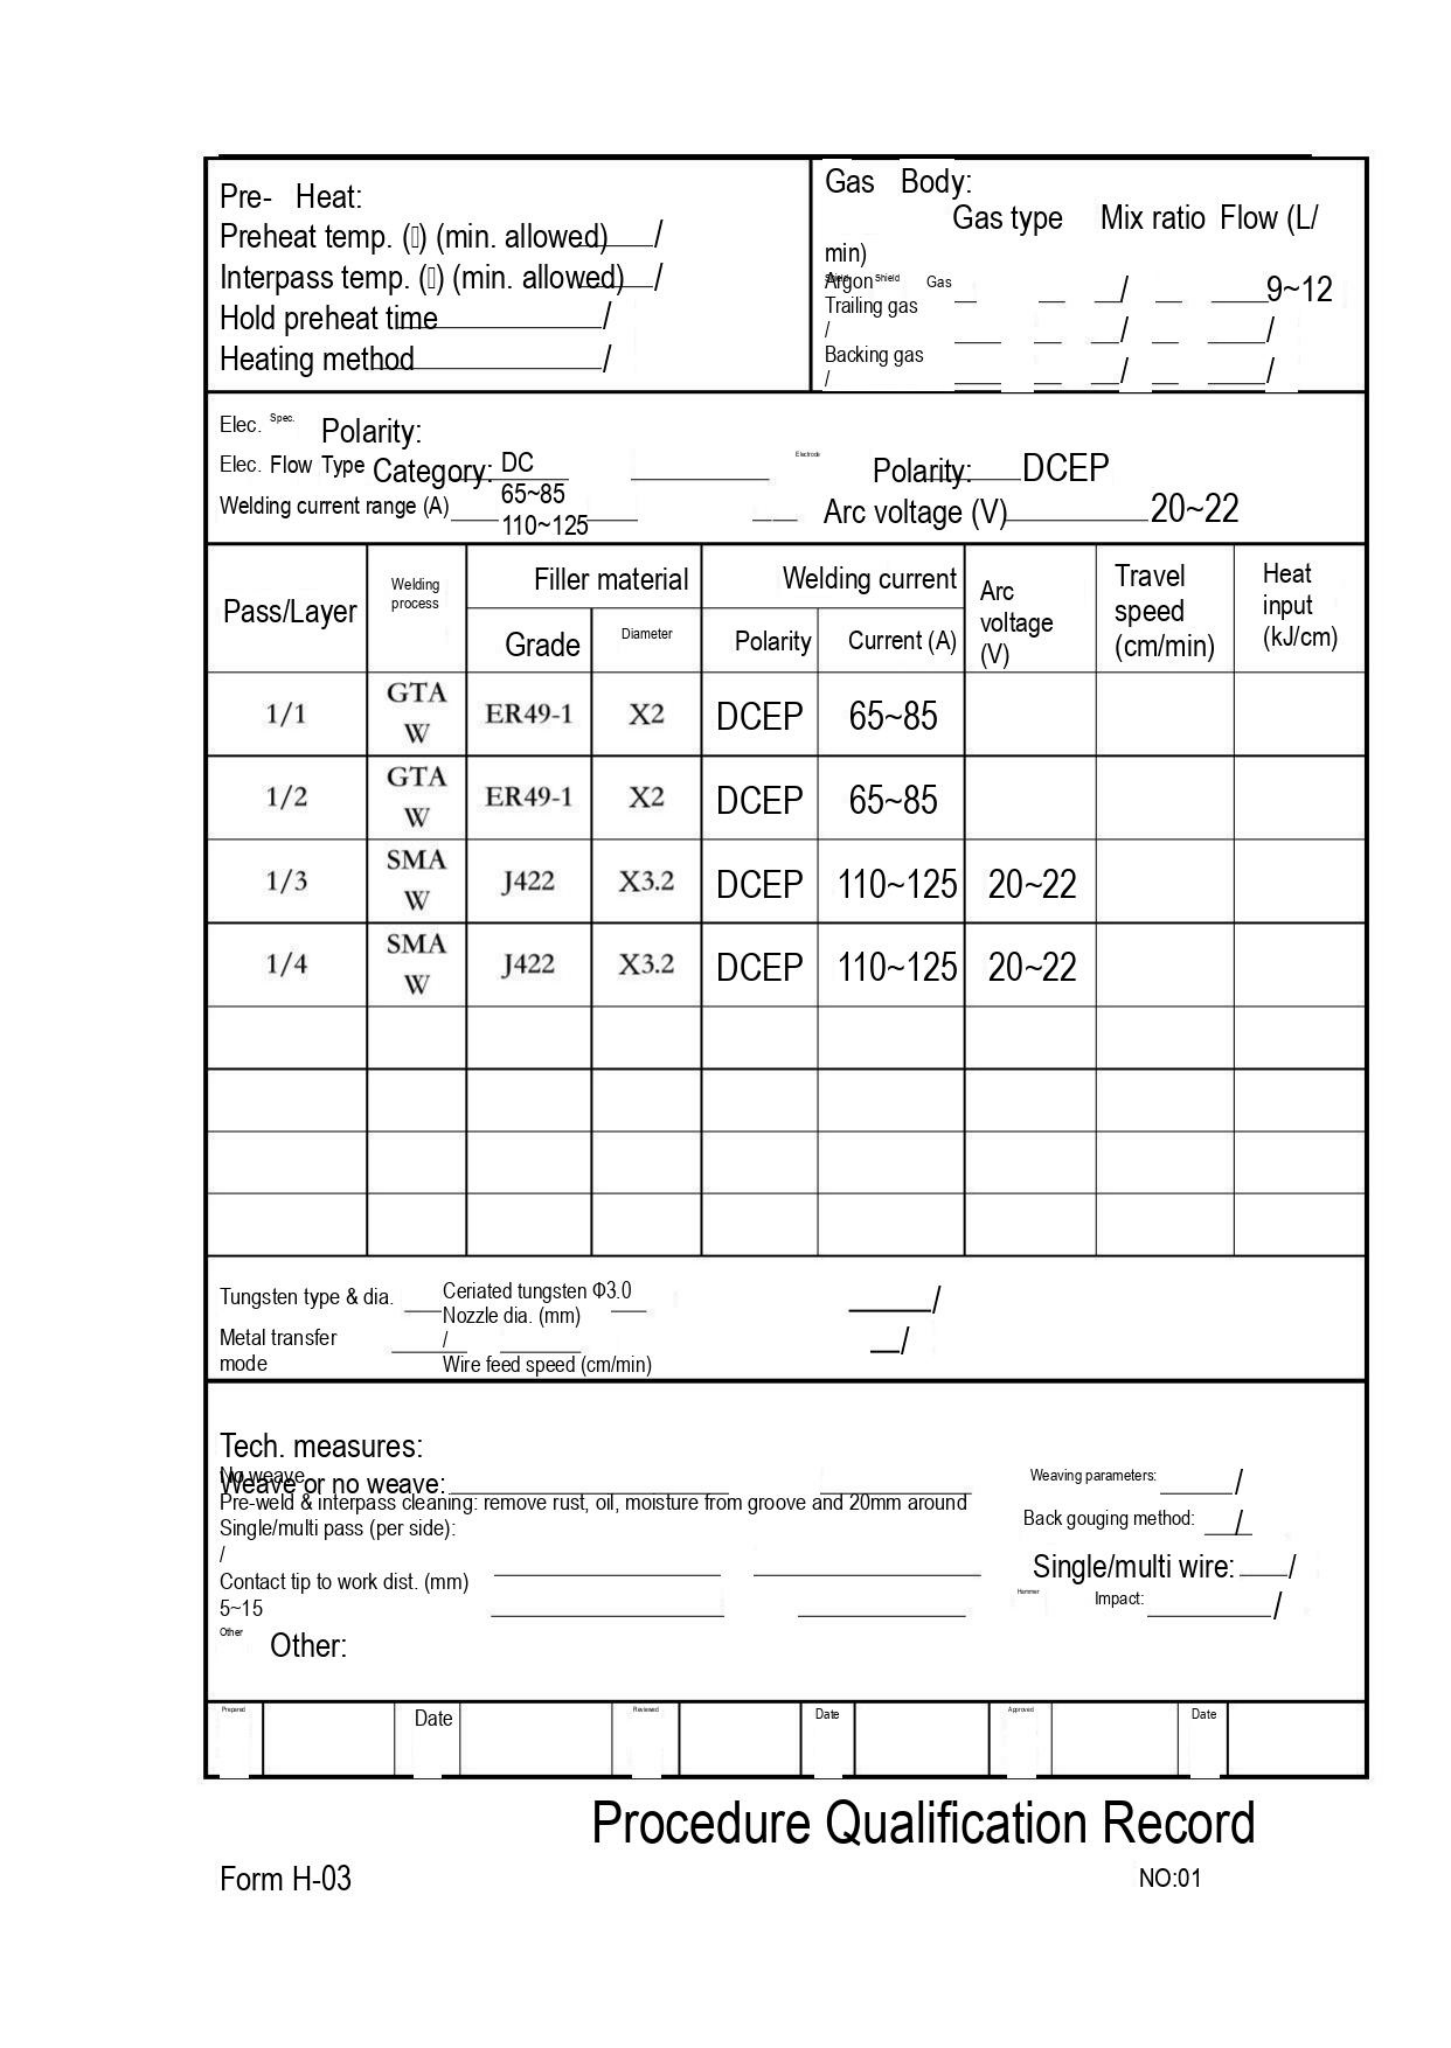Pre- Heat:
Preheat temp. (□) (min. allowed) /
Interpass temp. (□) (min. allowed) /
Hold preheat time /
Heating method /

Gas Body:
Gas type Mix ratio Flow (L/min)
Shield Argon Shield Gas / 9~12
Trailing gas / / /
Backing gas / / /

Elec. Spec. Polarity:
Elec. Flow Type Category: DC Electrode Polarity: DCEP
Welding current range (A) 65~85 110~125 Arc voltage (V) 20~22

| Pass/Layer | Welding process | Filler material Grade | Filler material Diameter | Welding current Polarity | Welding current Current (A) | Arc voltage (V) | Travel speed (cm/min) | Heat input (kJ/cm) |
|---|---|---|---|---|---|---|---|---|
| 1/1 | GTAW | ER49-1 | X2 | DCEP | 65~85 | | | |
| 1/2 | GTAW | ER49-1 | X2 | DCEP | 65~85 | | | |
| 1/3 | SMAW | J422 | X3.2 | DCEP | 110~125 | 20~22 | | |
| 1/4 | SMAW | J422 | X3.2 | DCEP | 110~125 | 20~22 | | |
| | | | | | | | | |
| | | | | | | | | |
| | | | | | | | | |
| | | | | | | | | |

Tungsten type & dia. Ceriated tungsten Φ3.0 Nozzle dia. (mm) /
Metal transfer mode / Wire feed speed (cm/min) /

Tech. measures:
No weave Weave or no weave:
Pre-weld & interpass cleaning: remove rust, oil, moisture from groove and 20mm around
Single/multi pass (per side):
/
Contact tip to work dist. (mm)
5~15
Weaving parameters: /
Back gouging method: /
Single/multi wire: /
Hammer Impact: /
Other Other:

| Prepared | | Date | | Reviewed | | Date | | Approved | | Date | |
|---|---|---|---|---|---|---|---|---|---|---|---|

Procedure Qualification Record
Form H-03
NO:01
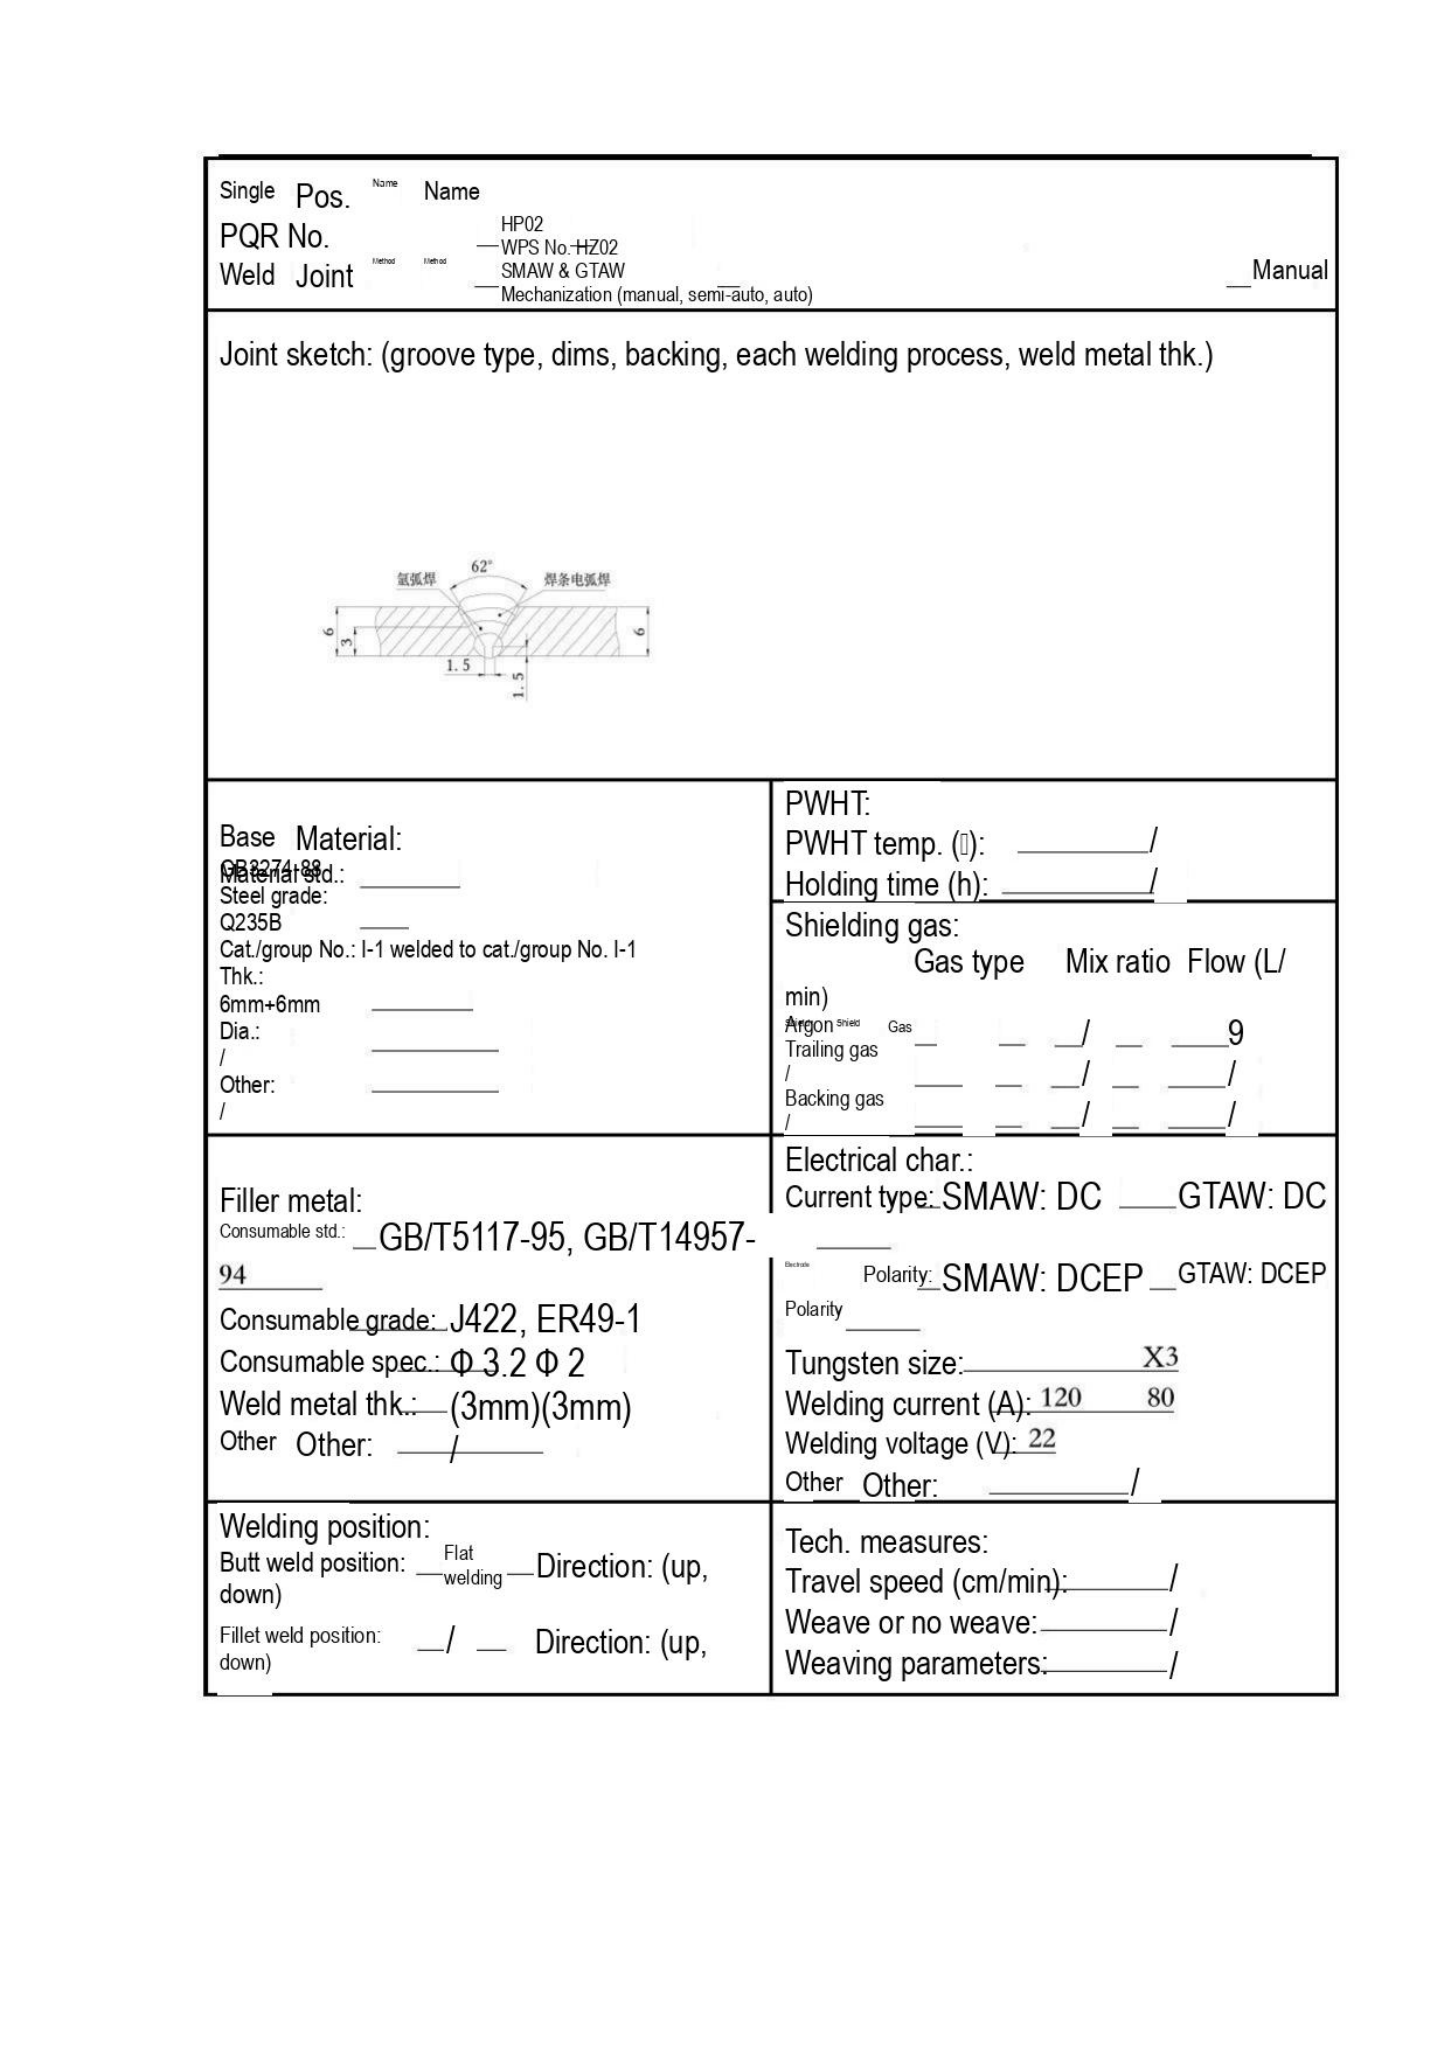Single Pos. Name Name
PQR No. HP02
WPS No. HZ02
Weld Joint Method Method SMAW & GTAW
Mechanization (manual, semi-auto, auto) Manual

Joint sketch: (groove type, dims, backing, each welding process, weld metal thk.)

氩弧焊 62° 焊条电弧焊
6 3 6
1.5 1.5

| | |
|---|---|
| Base Material:<br>Material std.: GB3274-88<br>Steel grade:<br>Q235B<br>Cat./group No.: I-1 welded to cat./group No. I-1<br>Thk.:<br>6mm+6mm<br>Dia.:<br>/<br>Other:<br>/ | PWHT:<br>PWHT temp. (): /<br>Holding time (h): / |
| | Shielding gas:<br>Gas type Mix ratio Flow (L/min)<br>Shield Gas Argon / 9<br>Trailing gas<br>/ / /<br>Backing gas<br>/ / / |
| Filler metal:<br>Consumable std.: GB/T5117-95, GB/T14957-94<br>Consumable grade: J422, ER49-1<br>Consumable spec.: Φ3.2 Φ2<br>Weld metal thk.: (3mm)(3mm)<br>Other Other: / | Electrical char.:<br>Current type: SMAW: DC GTAW: DC<br>Polarity: SMAW: DCEP GTAW: DCEP<br>Polarity<br>Tungsten size: X3<br>Welding current (A): 120 80<br>Welding voltage (V): 22<br>Other Other: / |
| Welding position:<br>Butt weld position: Flat welding Direction: (up, down)<br>Fillet weld position: / Direction: (up, down) | Tech. measures:<br>Travel speed (cm/min): /<br>Weave or no weave: /<br>Weaving parameters: / |
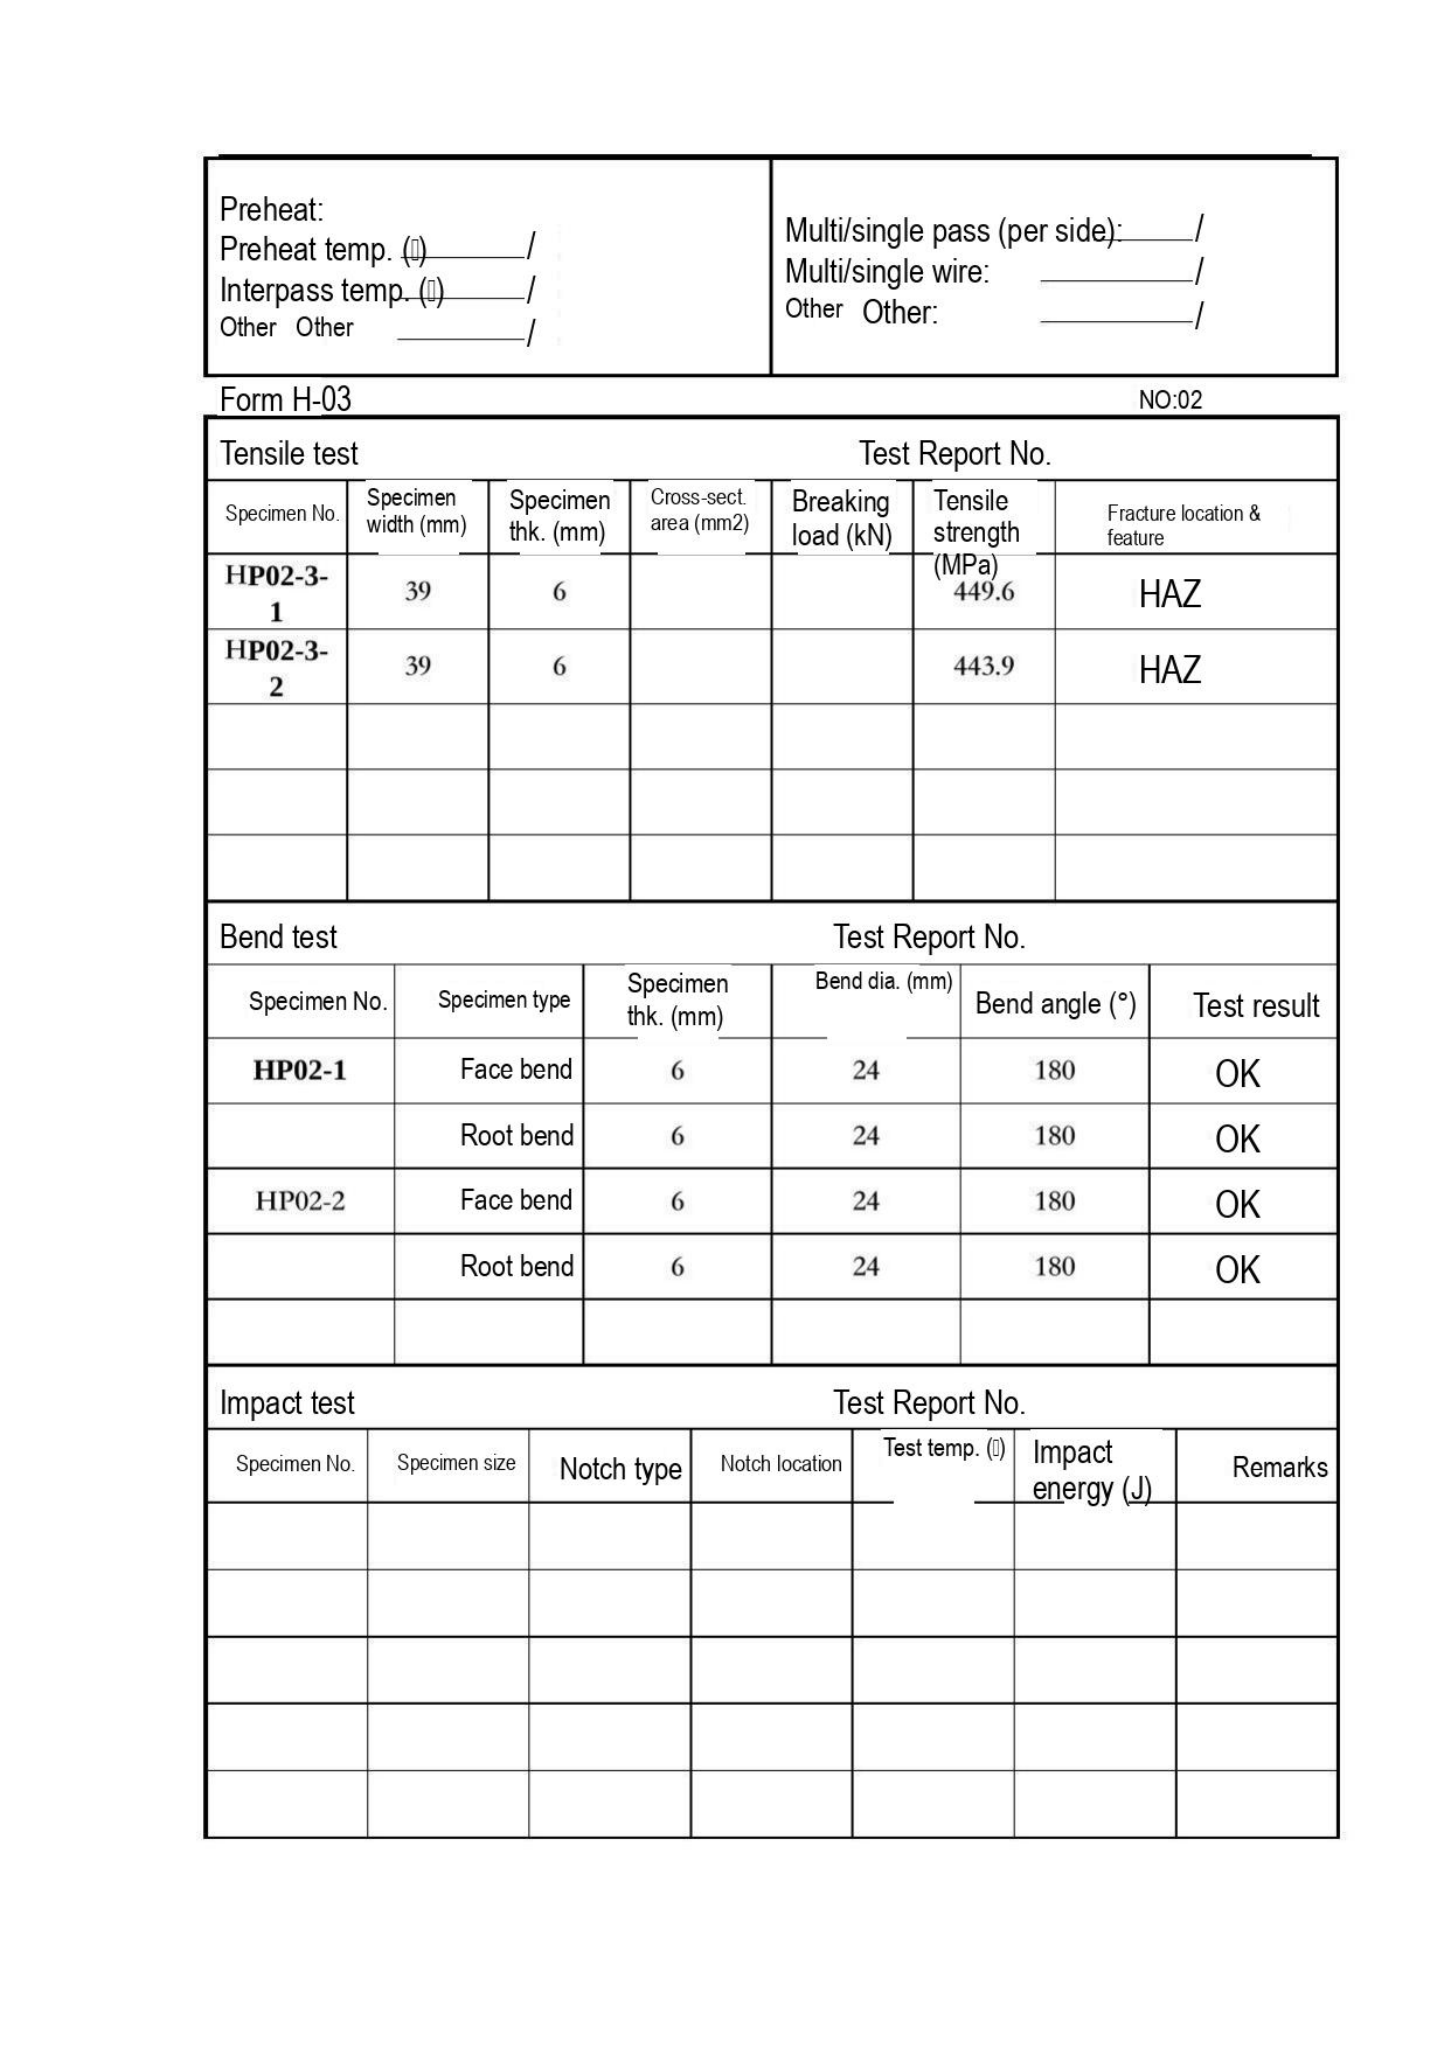Preheat:
Preheat temp. () /
Interpass temp. () /
Other Other /

Multi/single pass (per side): /
Multi/single wire: /
Other Other: /

Form H-03 NO:02

Tensile test Test Report No.

| Specimen No. | Specimen width (mm) | Specimen thk. (mm) | Cross-sect. area (mm2) | Breaking load (kN) | Tensile strength (MPa) | Fracture location & feature |
|---|---|---|---|---|---|---|
| HP02-3-1 | 39 | 6 | | | 449.6 | HAZ |
| HP02-3-2 | 39 | 6 | | | 443.9 | HAZ |
| | | | | | | |
| | | | | | | |
| | | | | | | |

Bend test Test Report No.

| Specimen No. | Specimen type | Specimen thk. (mm) | Bend dia. (mm) | Bend angle (°) | Test result |
|---|---|---|---|---|---|
| HP02-1 | Face bend | 6 | 24 | 180 | OK |
| | Root bend | 6 | 24 | 180 | OK |
| HP02-2 | Face bend | 6 | 24 | 180 | OK |
| | Root bend | 6 | 24 | 180 | OK |
| | | | | | |

Impact test Test Report No.

| Specimen No. | Specimen size | Notch type | Notch location | Test temp. () | Impact energy (J) | Remarks |
|---|---|---|---|---|---|---|
| | | | | | | |
| | | | | | | |
| | | | | | | |
| | | | | | | |
| | | | | | | |
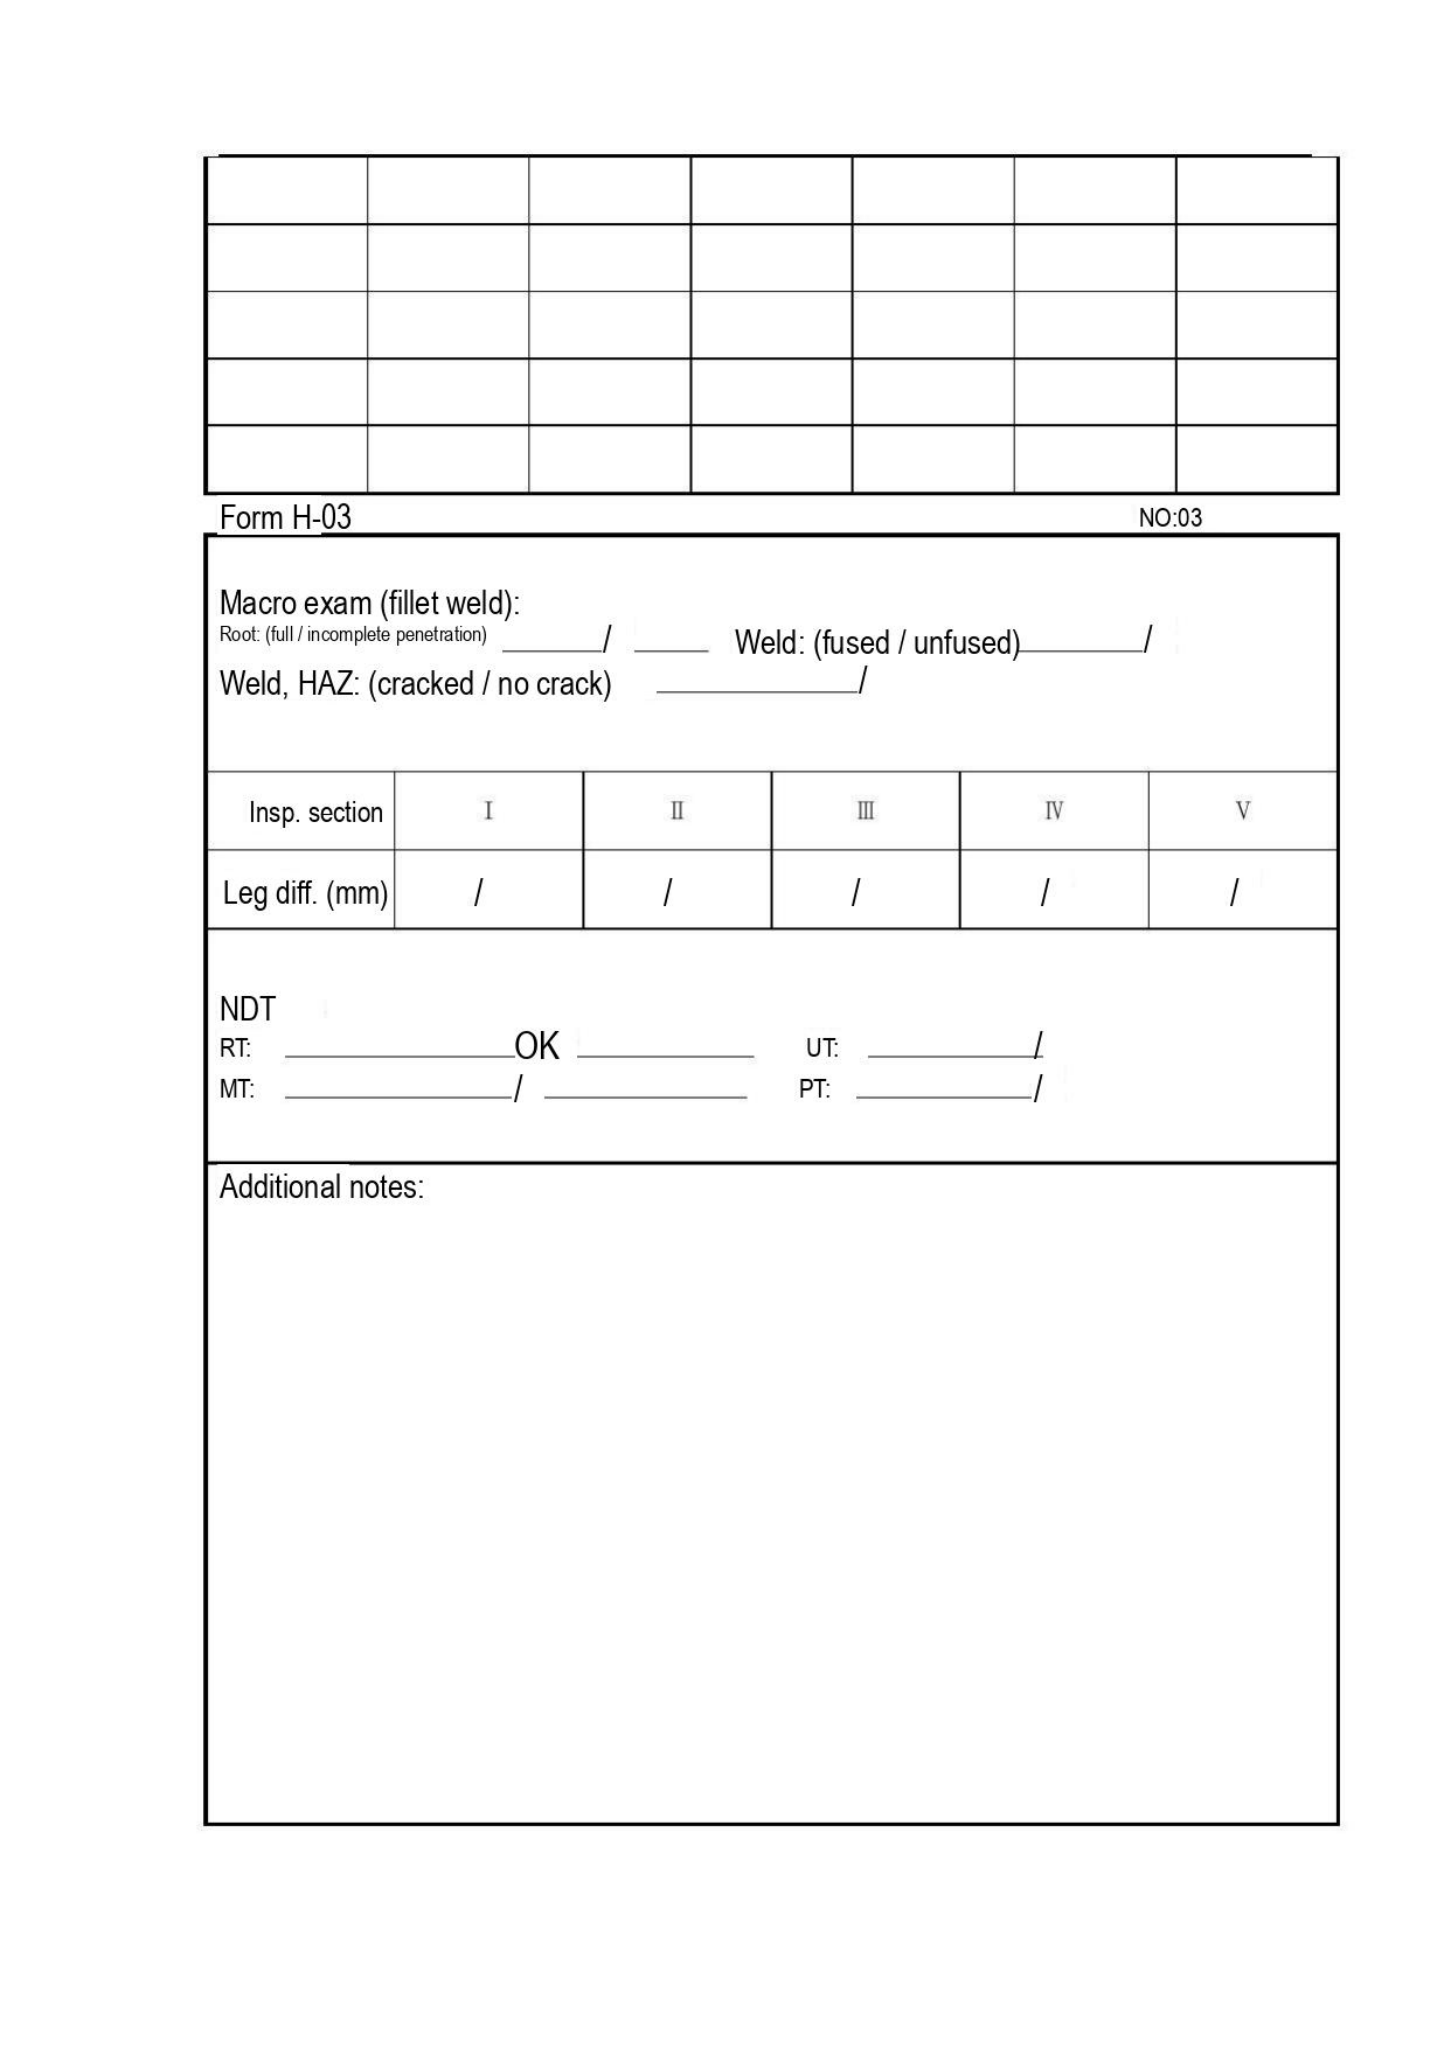|   |   |   |   |   |   |   |
|---|---|---|---|---|---|---|
|   |   |   |   |   |   |   |
|   |   |   |   |   |   |   |
|   |   |   |   |   |   |   |
|   |   |   |   |   |   |   |

Form H-03 NO:03

Macro exam (fillet weld):
Root: (full / incomplete penetration) ________/ ______ Weld: (fused / unfused)________/
Weld, HAZ: (cracked / no crack) ______________/

| Insp. section | I | II | III | IV | V |
|---|---|---|---|---|---|
| Leg diff. (mm) | / | / | / | / | / |

NDT
RT: ________________OK ______________ UT: ____________/
MT: ________________/ ______________ PT: ____________/

Additional notes:
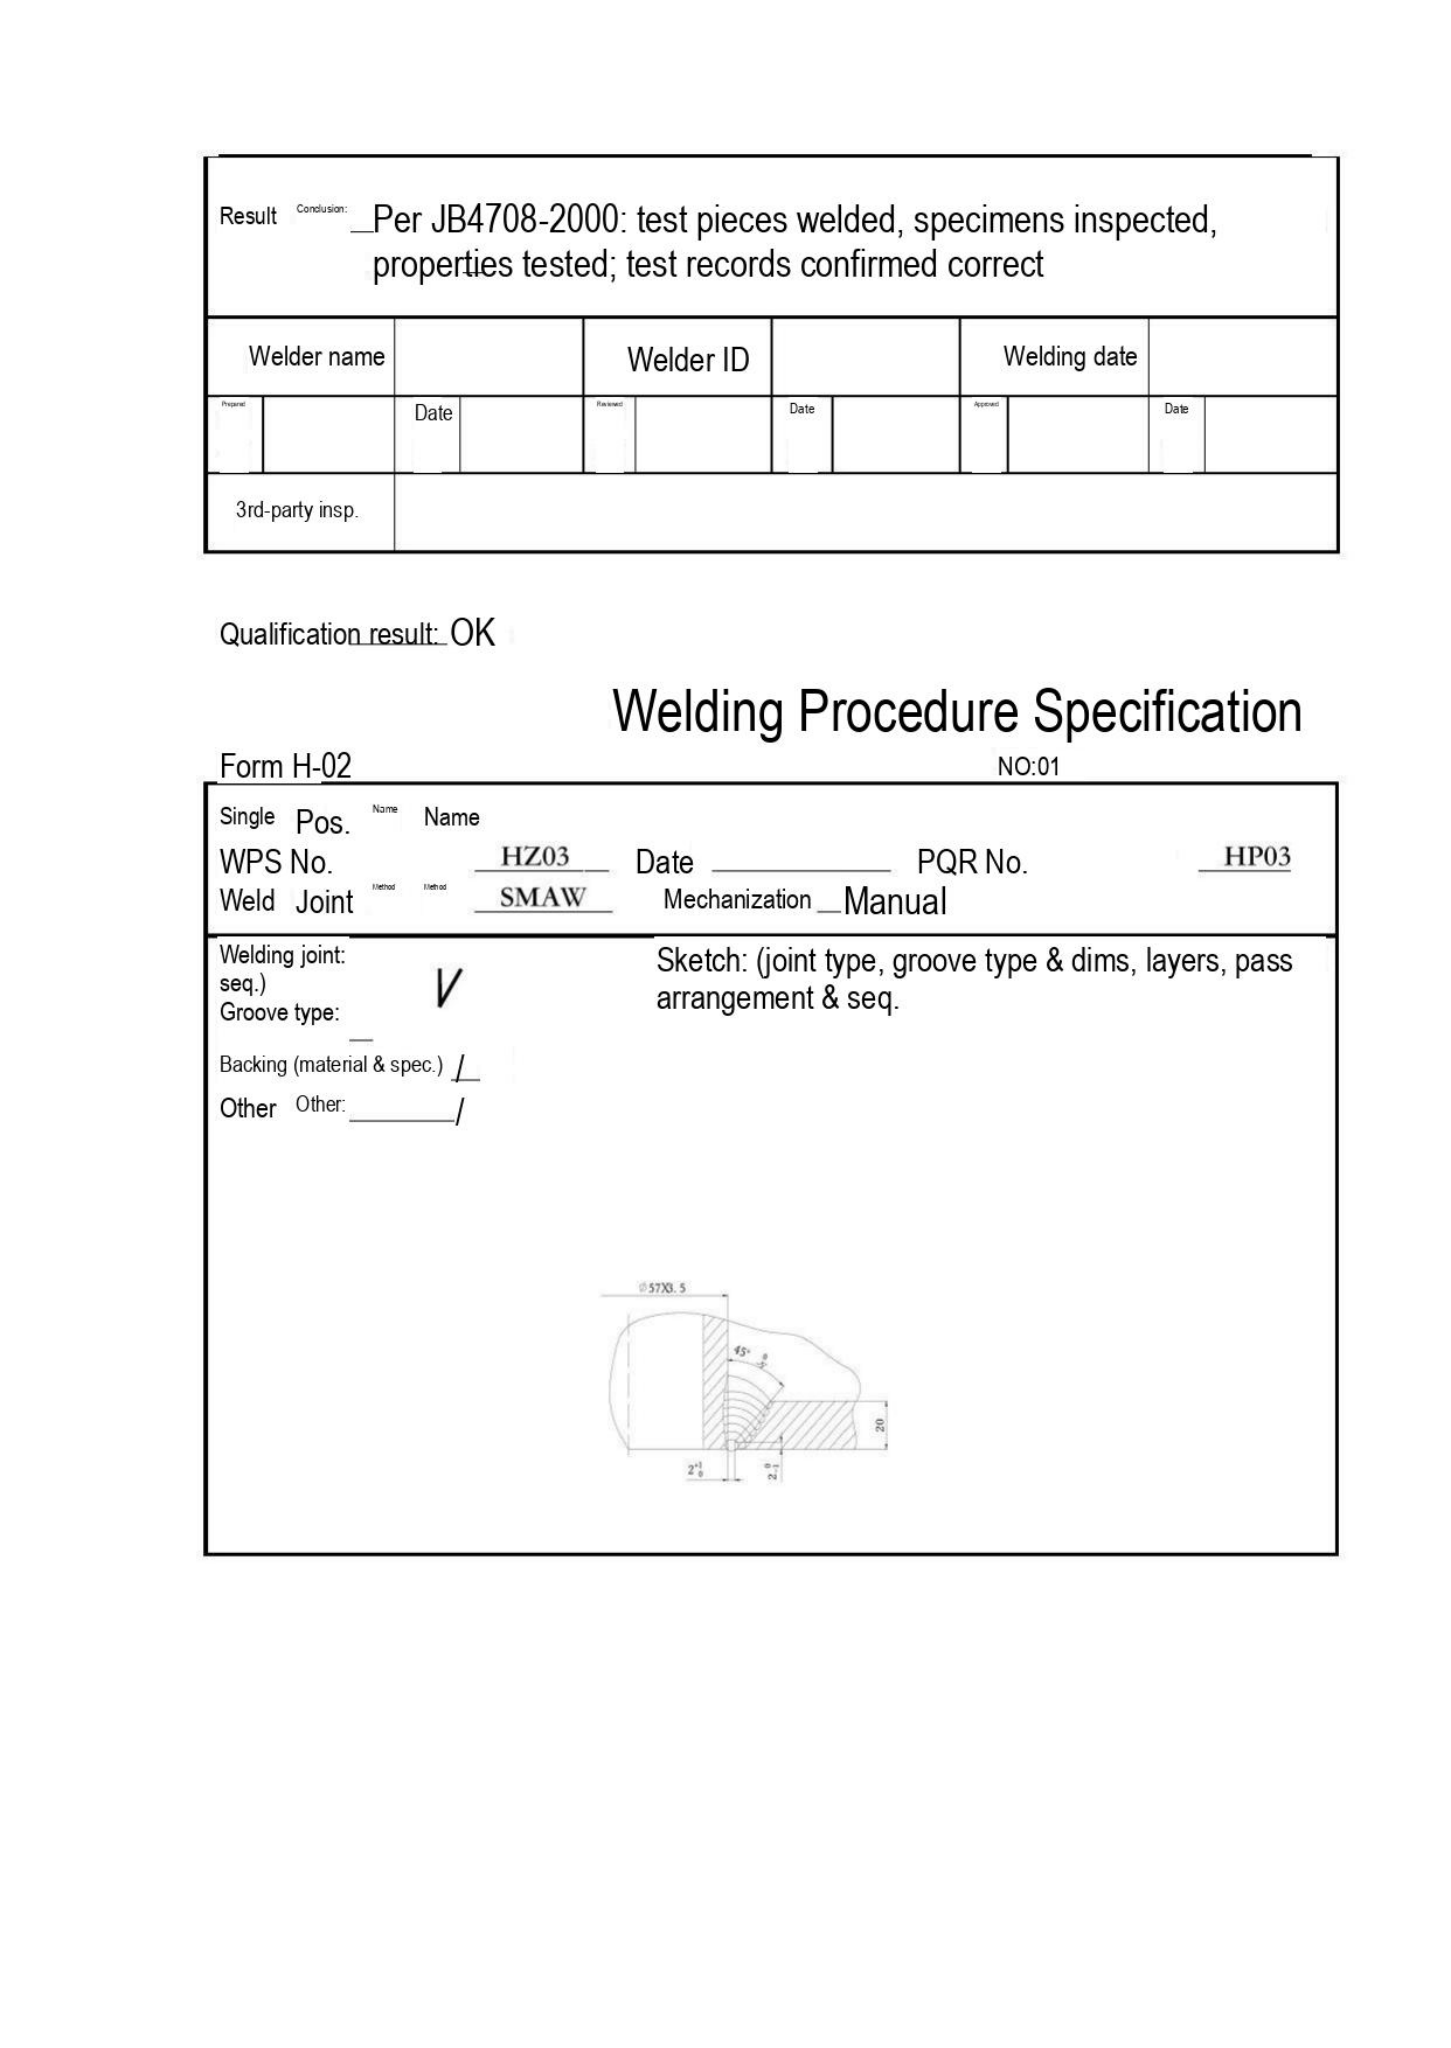| Result Conclusion: Per JB4708-2000: test pieces welded, specimens inspected, properties tested; test records confirmed correct | | | | | | | | | |
|---|---|---|---|---|---|---|---|---|---|
| Welder name | | Welder ID | | | | Welding date | | | |
| Prepared | | Date | | Reviewed | Date | | Approved | Date | |
| 3rd-party insp. | | | | | | | | | |

Qualification result: OK

Welding Procedure Specification

Form H-02

NO:01

Single Pos. Name Name
WPS No. HZ03 Date PQR No. HP03
Weld Joint Method Method SMAW Mechanization Manual

Welding joint:
seq.)
Groove type: V
Backing (material & spec.) /
Other Other: /

Sketch: (joint type, groove type & dims, layers, pass arrangement & seq.

Φ57X3.5
45°
20
2⁺¹₀
2⁰₋₁
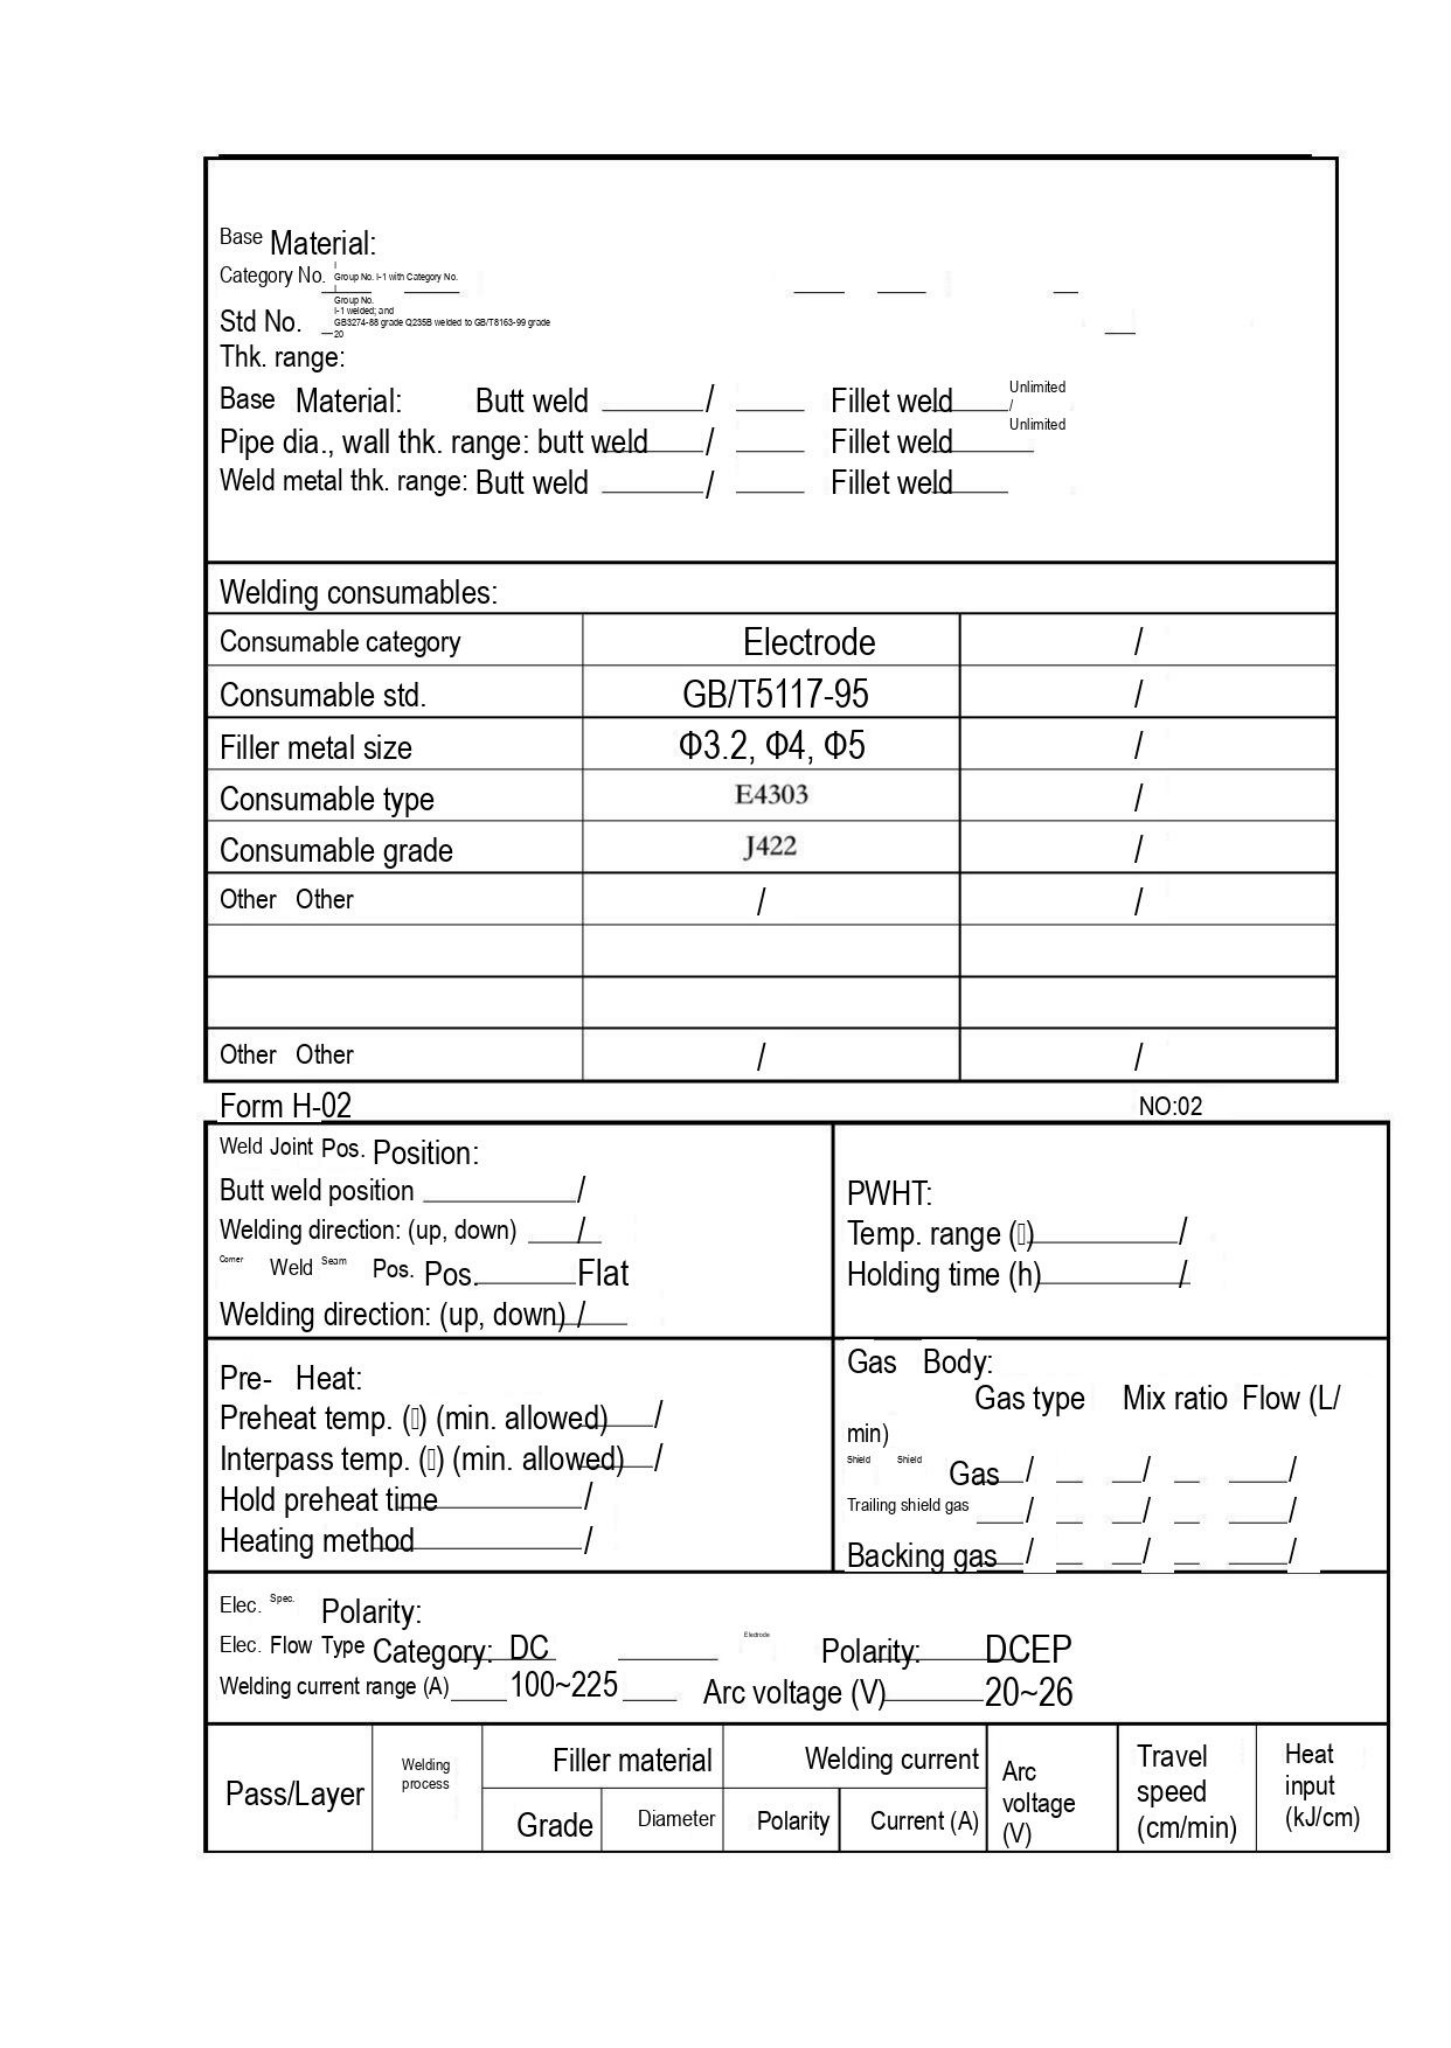Base Material:
Category No. Group No. I-1 with Category No.
Group No.
I-1 welded; and
Std No. GB3274-88 grade Q235B welded to GB/T8163-99 grade
20
Thk. range:
Base Material: Butt weld / Fillet weld Unlimited /
Pipe dia., wall thk. range: butt weld / Fillet weld Unlimited
Weld metal thk. range: Butt weld / Fillet weld

Welding consumables:

| Consumable category | Electrode | / |
|---|---|---|
| Consumable std. | GB/T5117-95 | / |
| Filler metal size | Φ3.2, Φ4, Φ5 | / |
| Consumable type | E4303 | / |
| Consumable grade | J422 | / |
| Other Other | / | / |
| | | |
| | | |
| Other Other | / | / |

Form H-02 NO:02

| Weld Joint Pos. Position:<br>Butt weld position /<br>Welding direction: (up, down) /<br>Corner Weld Seam Pos. Pos. Flat<br>Welding direction: (up, down) / | PWHT:<br>Temp. range () /<br>Holding time (h) / |
|---|---|
| Pre- Heat:<br>Preheat temp. () (min. allowed) /<br>Interpass temp. () (min. allowed) /<br>Hold preheat time /<br>Heating method / | Gas Body:<br>Gas type Mix ratio Flow (L/min)<br>Shield Shield Gas / / /<br>Trailing shield gas / / /<br>Backing gas / / / |

Elec. Spec. Polarity:
Elec. Flow Type Category: DC Electrode Polarity: DCEP
Welding current range (A) 100~225 Arc voltage (V) 20~26

| Pass/Layer | Welding process | Filler material: Grade | Filler material: Diameter | Welding current: Polarity | Welding current: Current (A) | Arc voltage (V) | Travel speed (cm/min) | Heat input (kJ/cm) |
|---|---|---|---|---|---|---|---|---|
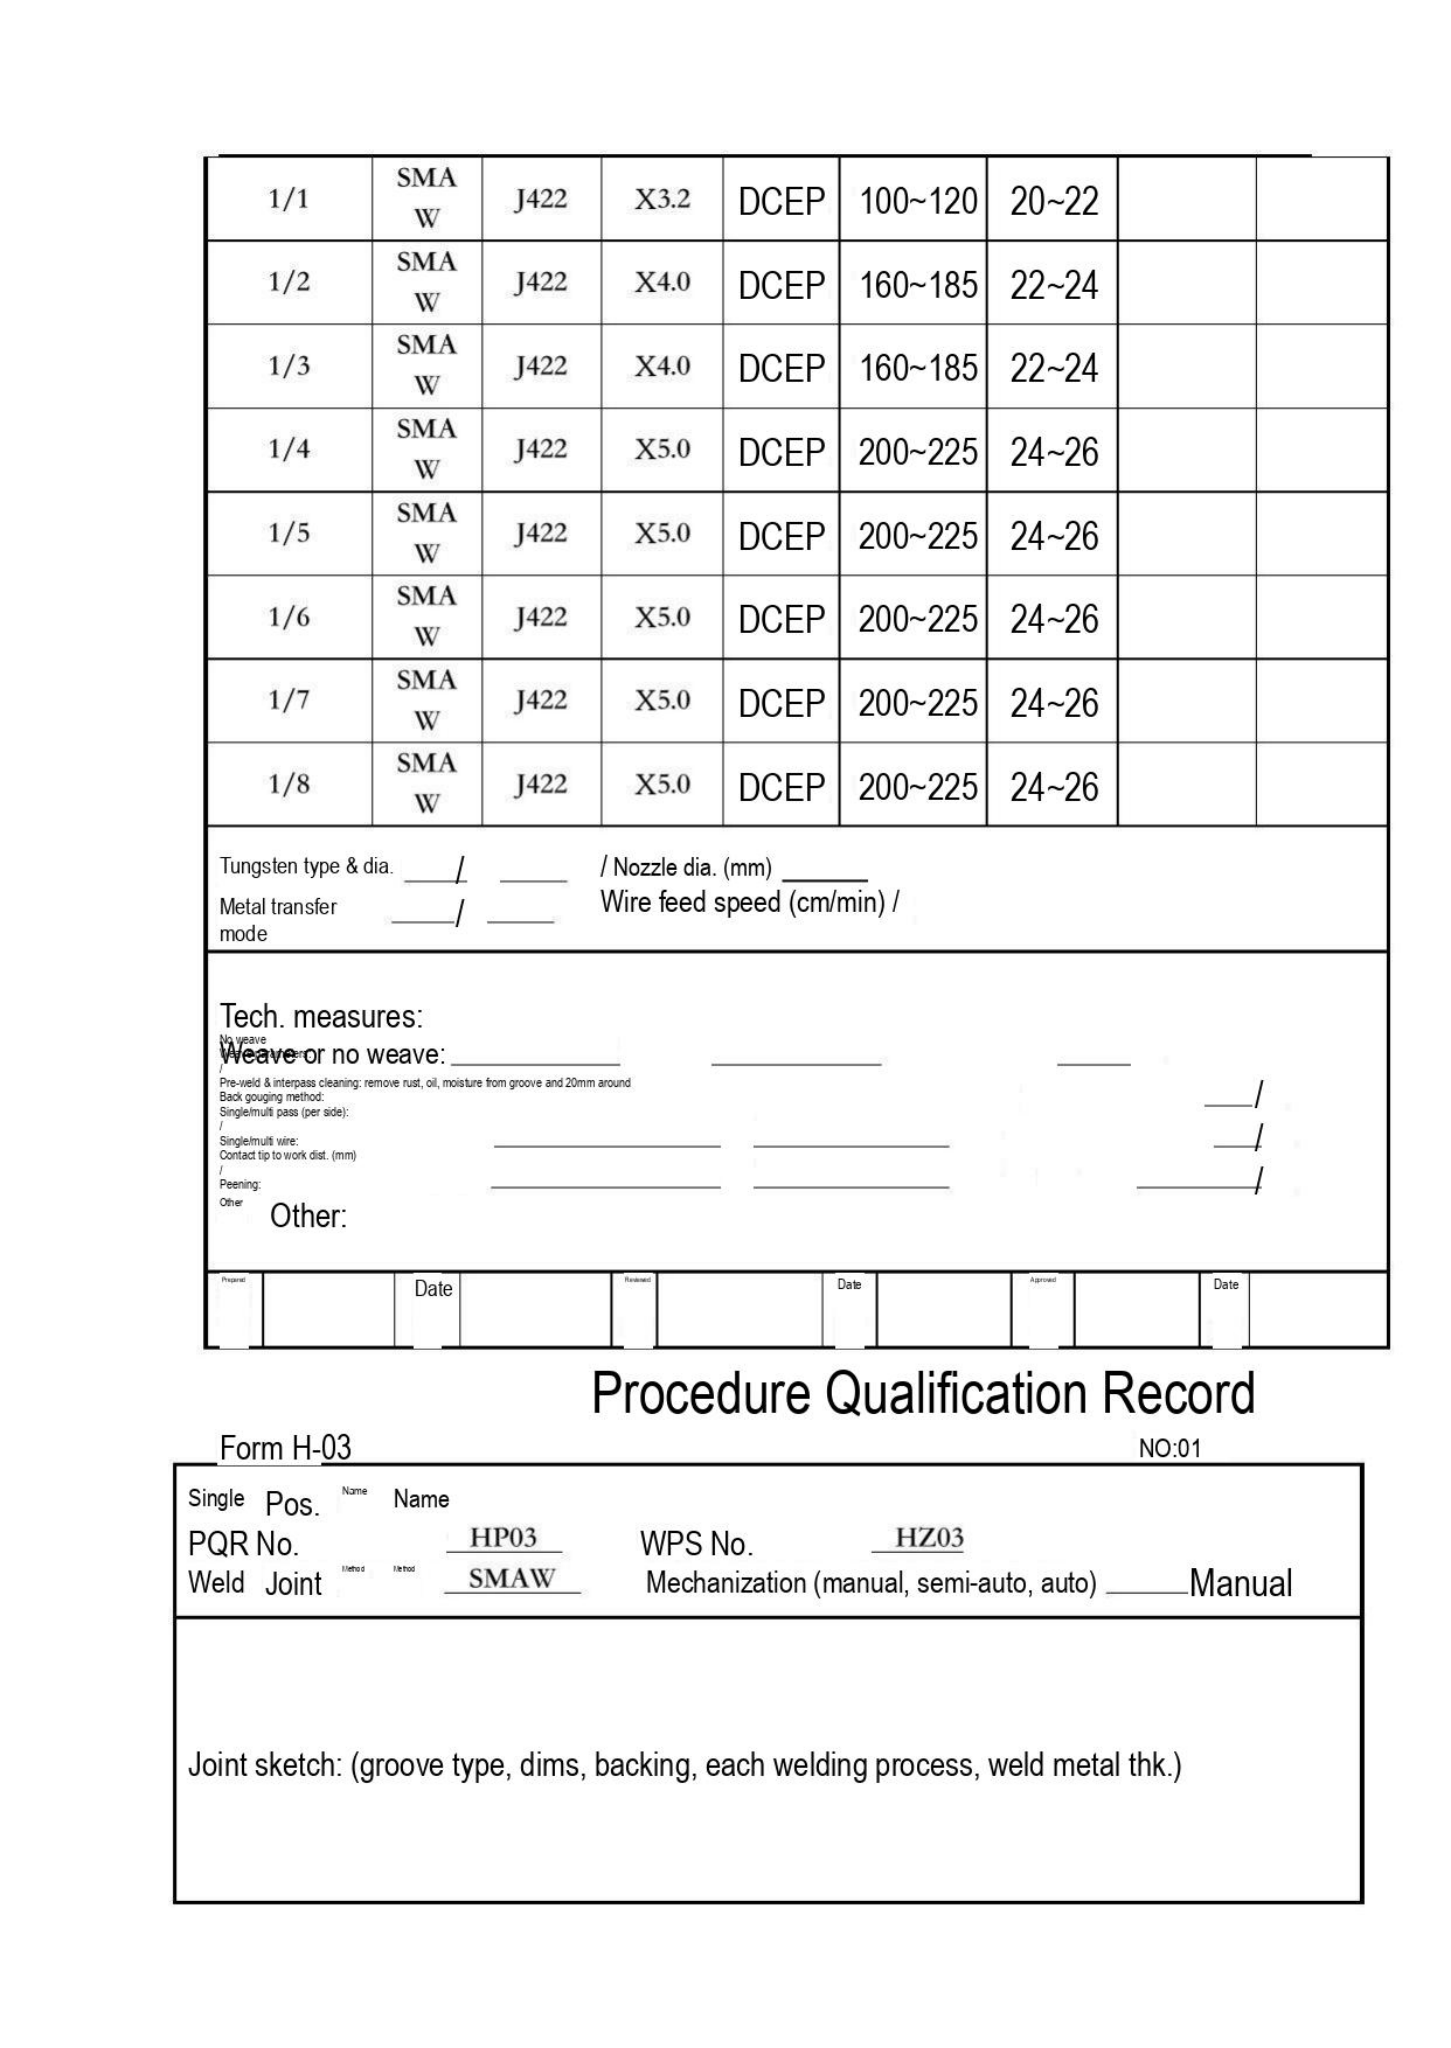| 1/1 | SMA W | J422 | X3.2 | DCEP | 100~120 | 20~22 | | |
|---|---|---|---|---|---|---|---|---|
| 1/2 | SMA W | J422 | X4.0 | DCEP | 160~185 | 22~24 | | |
| 1/3 | SMA W | J422 | X4.0 | DCEP | 160~185 | 22~24 | | |
| 1/4 | SMA W | J422 | X5.0 | DCEP | 200~225 | 24~26 | | |
| 1/5 | SMA W | J422 | X5.0 | DCEP | 200~225 | 24~26 | | |
| 1/6 | SMA W | J422 | X5.0 | DCEP | 200~225 | 24~26 | | |
| 1/7 | SMA W | J422 | X5.0 | DCEP | 200~225 | 24~26 | | |
| 1/8 | SMA W | J422 | X5.0 | DCEP | 200~225 | 24~26 | | |

Tungsten type & dia. ____/ ____ / Nozzle dia. (mm) ______
Metal transfer mode ____/ ____ Wire feed speed (cm/min) /

Tech. measures:
No weave
Weave or no weave: ____________ ____________ _____
/
Pre-weld & interpass cleaning: remove rust, oil, moisture from groove and 20mm around
Back gouging method:
Single/multi pass (per side):
/ ____/
Single/multi wire: ____________ ____________ ____/
Contact tip to work dist. (mm)
/
Peening: ____________ ____________ ________/
Other
Other:

| Prepared | | Date | | Reviewed | | Date | | Approved | | Date | |
|---|---|---|---|---|---|---|---|---|---|---|---|

Procedure Qualification Record

Form H-03 NO:01

Single Pos. Name Name
PQR No. HP03 WPS No. HZ03
Weld Joint Method Method SMAW Mechanization (manual, semi-auto, auto) ______Manual

Joint sketch: (groove type, dims, backing, each welding process, weld metal thk.)